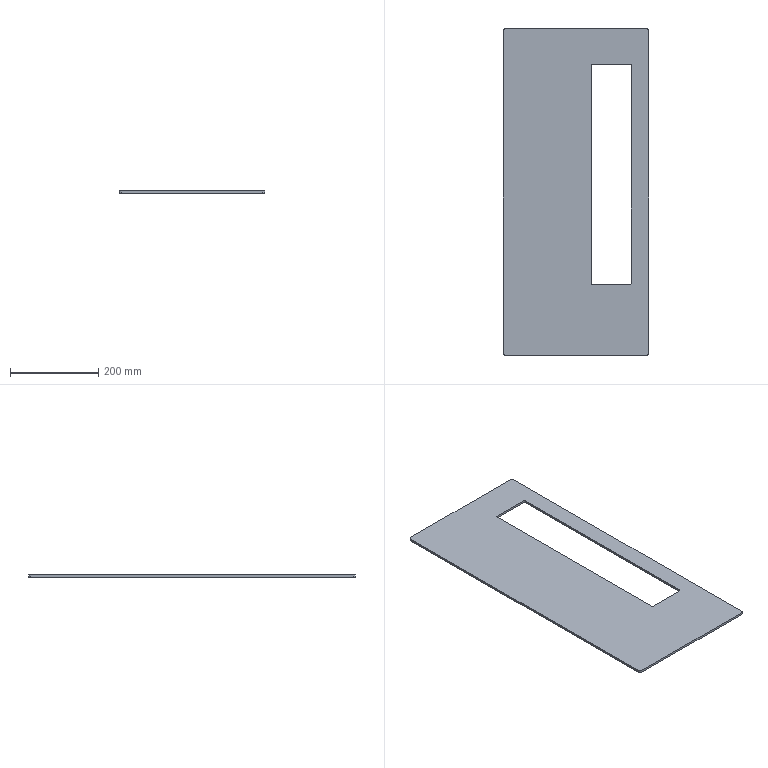Part | STEP file | 001-002-Face Plate-4 | 1 solid | 18 faces | box 330 x 740 x 5 mm | volume 995931 mm3 | plane 10 | cylinder 8 | commonest cylinder face diameters 6 x4 10 x4
STEP:
#1=CARTESIAN_POINT('',(0.,0.,0.));
#2=DIRECTION('',(0.,0.,1.));
#3=DIRECTION('',(1.,0.,0.));
#4=AXIS2_PLACEMENT_3D('',#1,#2,#3);
#5=CARTESIAN_POINT('',(165.,-365.,0.));
#6=VERTEX_POINT('',#5);
#7=CARTESIAN_POINT('',(165.,365.,0.));
#8=VERTEX_POINT('',#7);
#9=CARTESIAN_POINT('',(165.,-370.,0.));
#10=DIRECTION('',(0.,1.,0.));
#11=VECTOR('',#10,1.);
#12=LINE('',#9,#11);
#13=CARTESIAN_POINT('',(165.,-370.,5.));
#14=DIRECTION('',(-1.,0.,0.));
#15=DIRECTION('',(0.,0.,1.));
#16=AXIS2_PLACEMENT_3D('',#13,#14,#15);
#17=PLANE('',#16);
#18=CARTESIAN_POINT('',(-5.,0.));
#19=DIRECTION('',(0.,1.));
#20=VECTOR('',#19,1.);
#21=LINE('',#18,#20);
#22=(GEOMETRIC_REPRESENTATION_CONTEXT(2)PARAMETRIC_REPRESENTATION_CONTEXT()REPRESENTATION_CONTEXT('',''));
#23=DEFINITIONAL_REPRESENTATION('',(#21),#22);
#24=PCURVE('',#17,#23);
#25=CARTESIAN_POINT('',(0.,0.,0.));
#26=DIRECTION('',(0.,0.,-1.));
#27=DIRECTION('',(-1.,0.,0.));
#28=AXIS2_PLACEMENT_3D('',#25,#26,#27);
#29=PLANE('',#28);
#30=CARTESIAN_POINT('',(-165.,-370.));
#31=DIRECTION('',(0.,1.));
#32=VECTOR('',#31,1.);
#33=LINE('',#30,#32);
#34=(GEOMETRIC_REPRESENTATION_CONTEXT(2)PARAMETRIC_REPRESENTATION_CONTEXT()REPRESENTATION_CONTEXT('',''));
#35=DEFINITIONAL_REPRESENTATION('',(#33),#34);
#36=PCURVE('',#29,#35);
#37=SURFACE_CURVE('',#12,(#24,#36),.PCURVE_S1.);
#38=EDGE_CURVE('',#6,#8,#37,.T.);
#39=ORIENTED_EDGE('',*,*,#38,.T.);
#40=CARTESIAN_POINT('',(165.,365.,5.));
#41=VERTEX_POINT('',#40);
#42=CARTESIAN_POINT('',(165.,365.,5.));
#43=DIRECTION('',(0.,0.,1.));
#44=VECTOR('',#43,1.);
#45=LINE('',#42,#44);
#46=CARTESIAN_POINT('',(0.,735.));
#47=DIRECTION('',(1.,0.));
#48=VECTOR('',#47,1.);
#49=LINE('',#46,#48);
#50=(GEOMETRIC_REPRESENTATION_CONTEXT(2)PARAMETRIC_REPRESENTATION_CONTEXT()REPRESENTATION_CONTEXT('',''));
#51=DEFINITIONAL_REPRESENTATION('',(#49),#50);
#52=PCURVE('',#17,#51);
#53=CARTESIAN_POINT('',(160.,365.,5.));
#54=DIRECTION('',(0.,0.,-1.));
#55=DIRECTION('',(-1.,0.,0.));
#56=AXIS2_PLACEMENT_3D('',#53,#54,#55);
#57=CYLINDRICAL_SURFACE('',#56,5.);
#58=CARTESIAN_POINT('',(3.142,0.));
#59=DIRECTION('',(0.,-1.));
#60=VECTOR('',#59,1.);
#61=LINE('',#58,#60);
#62=(GEOMETRIC_REPRESENTATION_CONTEXT(2)PARAMETRIC_REPRESENTATION_CONTEXT()REPRESENTATION_CONTEXT('',''));
#63=DEFINITIONAL_REPRESENTATION('',(#61),#62);
#64=PCURVE('',#57,#63);
#65=SURFACE_CURVE('',#45,(#52,#64),.PCURVE_S1.);
#66=EDGE_CURVE('',#8,#41,#65,.T.);
#67=ORIENTED_EDGE('',*,*,#66,.T.);
#68=CARTESIAN_POINT('',(165.,-365.,5.));
#69=VERTEX_POINT('',#68);
#70=CARTESIAN_POINT('',(165.,-370.,5.));
#71=DIRECTION('',(0.,1.,0.));
#72=VECTOR('',#71,1.);
#73=LINE('',#70,#72);
#74=CARTESIAN_POINT('',(0.,0.));
#75=DIRECTION('',(0.,1.));
#76=VECTOR('',#75,1.);
#77=LINE('',#74,#76);
#78=(GEOMETRIC_REPRESENTATION_CONTEXT(2)PARAMETRIC_REPRESENTATION_CONTEXT()REPRESENTATION_CONTEXT('',''));
#79=DEFINITIONAL_REPRESENTATION('',(#77),#78);
#80=PCURVE('',#17,#79);
#81=CARTESIAN_POINT('',(0.,0.,5.));
#82=DIRECTION('',(0.,0.,-1.));
#83=DIRECTION('',(-1.,0.,0.));
#84=AXIS2_PLACEMENT_3D('',#81,#82,#83);
#85=PLANE('',#84);
#86=CARTESIAN_POINT('',(-165.,-370.));
#87=DIRECTION('',(0.,1.));
#88=VECTOR('',#87,1.);
#89=LINE('',#86,#88);
#90=(GEOMETRIC_REPRESENTATION_CONTEXT(2)PARAMETRIC_REPRESENTATION_CONTEXT()REPRESENTATION_CONTEXT('',''));
#91=DEFINITIONAL_REPRESENTATION('',(#89),#90);
#92=PCURVE('',#85,#91);
#93=SURFACE_CURVE('',#73,(#80,#92),.PCURVE_S1.);
#94=EDGE_CURVE('',#69,#41,#93,.T.);
#95=ORIENTED_EDGE('',*,*,#94,.F.);
#96=CARTESIAN_POINT('',(165.,-365.,5.));
#97=DIRECTION('',(0.,0.,-1.));
#98=VECTOR('',#97,1.);
#99=LINE('',#96,#98);
#100=CARTESIAN_POINT('',(0.,5.));
#101=DIRECTION('',(-1.,0.));
#102=VECTOR('',#101,1.);
#103=LINE('',#100,#102);
#104=(GEOMETRIC_REPRESENTATION_CONTEXT(2)PARAMETRIC_REPRESENTATION_CONTEXT()REPRESENTATION_CONTEXT('',''));
#105=DEFINITIONAL_REPRESENTATION('',(#103),#104);
#106=PCURVE('',#17,#105);
#107=CARTESIAN_POINT('',(160.,-365.,5.));
#108=DIRECTION('',(0.,0.,-1.));
#109=DIRECTION('',(-1.,0.,0.));
#110=AXIS2_PLACEMENT_3D('',#107,#108,#109);
#111=CYLINDRICAL_SURFACE('',#110,5.);
#112=CARTESIAN_POINT('',(3.142,0.));
#113=DIRECTION('',(0.,1.));
#114=VECTOR('',#113,1.);
#115=LINE('',#112,#114);
#116=(GEOMETRIC_REPRESENTATION_CONTEXT(2)PARAMETRIC_REPRESENTATION_CONTEXT()REPRESENTATION_CONTEXT('',''));
#117=DEFINITIONAL_REPRESENTATION('',(#115),#116);
#118=PCURVE('',#111,#117);
#119=SURFACE_CURVE('',#99,(#106,#118),.PCURVE_S1.);
#120=EDGE_CURVE('',#69,#6,#119,.T.);
#121=ORIENTED_EDGE('',*,*,#120,.T.);
#122=EDGE_LOOP('',(#39,#67,#95,#121));
#123=FACE_BOUND('',#122,.T.);
#124=ADVANCED_FACE('',(#123),#17,.F.);
#125=CARTESIAN_POINT('',(160.,370.,0.));
#126=VERTEX_POINT('',#125);
#127=CARTESIAN_POINT('',(-160.,370.,0.));
#128=VERTEX_POINT('',#127);
#129=CARTESIAN_POINT('',(-165.,370.,0.));
#130=DIRECTION('',(-1.,0.,0.));
#131=VECTOR('',#130,1.);
#132=LINE('',#129,#131);
#133=CARTESIAN_POINT('',(-165.,370.,5.));
#134=DIRECTION('',(0.,-1.,0.));
#135=DIRECTION('',(0.,0.,-1.));
#136=AXIS2_PLACEMENT_3D('',#133,#134,#135);
#137=PLANE('',#136);
#138=CARTESIAN_POINT('',(5.,0.));
#139=DIRECTION('',(0.,-1.));
#140=VECTOR('',#139,1.);
#141=LINE('',#138,#140);
#142=(GEOMETRIC_REPRESENTATION_CONTEXT(2)PARAMETRIC_REPRESENTATION_CONTEXT()REPRESENTATION_CONTEXT('',''));
#143=DEFINITIONAL_REPRESENTATION('',(#141),#142);
#144=PCURVE('',#137,#143);
#145=CARTESIAN_POINT('',(165.,370.));
#146=DIRECTION('',(1.,0.));
#147=VECTOR('',#146,1.);
#148=LINE('',#145,#147);
#149=(GEOMETRIC_REPRESENTATION_CONTEXT(2)PARAMETRIC_REPRESENTATION_CONTEXT()REPRESENTATION_CONTEXT('',''));
#150=DEFINITIONAL_REPRESENTATION('',(#148),#149);
#151=PCURVE('',#29,#150);
#152=SURFACE_CURVE('',#132,(#144,#151),.PCURVE_S1.);
#153=EDGE_CURVE('',#126,#128,#152,.T.);
#154=ORIENTED_EDGE('',*,*,#153,.T.);
#155=CARTESIAN_POINT('',(-160.,370.,5.));
#156=VERTEX_POINT('',#155);
#157=CARTESIAN_POINT('',(-160.,370.,5.));
#158=DIRECTION('',(0.,0.,1.));
#159=VECTOR('',#158,1.);
#160=LINE('',#157,#159);
#161=CARTESIAN_POINT('',(0.,5.));
#162=DIRECTION('',(-1.,0.));
#163=VECTOR('',#162,1.);
#164=LINE('',#161,#163);
#165=(GEOMETRIC_REPRESENTATION_CONTEXT(2)PARAMETRIC_REPRESENTATION_CONTEXT()REPRESENTATION_CONTEXT('',''));
#166=DEFINITIONAL_REPRESENTATION('',(#164),#165);
#167=PCURVE('',#137,#166);
#168=CARTESIAN_POINT('',(-160.,365.,5.));
#169=DIRECTION('',(0.,0.,-1.));
#170=DIRECTION('',(-1.,0.,0.));
#171=AXIS2_PLACEMENT_3D('',#168,#169,#170);
#172=CYLINDRICAL_SURFACE('',#171,5.);
#173=CARTESIAN_POINT('',(1.571,0.));
#174=DIRECTION('',(0.,-1.));
#175=VECTOR('',#174,1.);
#176=LINE('',#173,#175);
#177=(GEOMETRIC_REPRESENTATION_CONTEXT(2)PARAMETRIC_REPRESENTATION_CONTEXT()REPRESENTATION_CONTEXT('',''));
#178=DEFINITIONAL_REPRESENTATION('',(#176),#177);
#179=PCURVE('',#172,#178);
#180=SURFACE_CURVE('',#160,(#167,#179),.PCURVE_S1.);
#181=EDGE_CURVE('',#128,#156,#180,.T.);
#182=ORIENTED_EDGE('',*,*,#181,.T.);
#183=CARTESIAN_POINT('',(160.,370.,5.));
#184=VERTEX_POINT('',#183);
#185=CARTESIAN_POINT('',(-165.,370.,5.));
#186=DIRECTION('',(-1.,0.,0.));
#187=VECTOR('',#186,1.);
#188=LINE('',#185,#187);
#189=CARTESIAN_POINT('',(0.,0.));
#190=DIRECTION('',(0.,-1.));
#191=VECTOR('',#190,1.);
#192=LINE('',#189,#191);
#193=(GEOMETRIC_REPRESENTATION_CONTEXT(2)PARAMETRIC_REPRESENTATION_CONTEXT()REPRESENTATION_CONTEXT('',''));
#194=DEFINITIONAL_REPRESENTATION('',(#192),#193);
#195=PCURVE('',#137,#194);
#196=CARTESIAN_POINT('',(165.,370.));
#197=DIRECTION('',(1.,0.));
#198=VECTOR('',#197,1.);
#199=LINE('',#196,#198);
#200=(GEOMETRIC_REPRESENTATION_CONTEXT(2)PARAMETRIC_REPRESENTATION_CONTEXT()REPRESENTATION_CONTEXT('',''));
#201=DEFINITIONAL_REPRESENTATION('',(#199),#200);
#202=PCURVE('',#85,#201);
#203=SURFACE_CURVE('',#188,(#195,#202),.PCURVE_S1.);
#204=EDGE_CURVE('',#184,#156,#203,.T.);
#205=ORIENTED_EDGE('',*,*,#204,.F.);
#206=CARTESIAN_POINT('',(160.,370.,5.));
#207=DIRECTION('',(0.,0.,-1.));
#208=VECTOR('',#207,1.);
#209=LINE('',#206,#208);
#210=CARTESIAN_POINT('',(0.,325.));
#211=DIRECTION('',(1.,0.));
#212=VECTOR('',#211,1.);
#213=LINE('',#210,#212);
#214=(GEOMETRIC_REPRESENTATION_CONTEXT(2)PARAMETRIC_REPRESENTATION_CONTEXT()REPRESENTATION_CONTEXT('',''));
#215=DEFINITIONAL_REPRESENTATION('',(#213),#214);
#216=PCURVE('',#137,#215);
#217=CARTESIAN_POINT('',(1.571,0.));
#218=DIRECTION('',(0.,1.));
#219=VECTOR('',#218,1.);
#220=LINE('',#217,#219);
#221=(GEOMETRIC_REPRESENTATION_CONTEXT(2)PARAMETRIC_REPRESENTATION_CONTEXT()REPRESENTATION_CONTEXT('',''));
#222=DEFINITIONAL_REPRESENTATION('',(#220),#221);
#223=PCURVE('',#57,#222);
#224=SURFACE_CURVE('',#209,(#216,#223),.PCURVE_S1.);
#225=EDGE_CURVE('',#184,#126,#224,.T.);
#226=ORIENTED_EDGE('',*,*,#225,.T.);
#227=EDGE_LOOP('',(#154,#182,#205,#226));
#228=FACE_BOUND('',#227,.T.);
#229=ADVANCED_FACE('',(#228),#137,.F.);
#230=CARTESIAN_POINT('',(-165.,365.,0.));
#231=VERTEX_POINT('',#230);
#232=CARTESIAN_POINT('',(-165.,-365.,0.));
#233=VERTEX_POINT('',#232);
#234=CARTESIAN_POINT('',(-165.,-370.,0.));
#235=DIRECTION('',(0.,-1.,0.));
#236=VECTOR('',#235,1.);
#237=LINE('',#234,#236);
#238=CARTESIAN_POINT('',(-165.,-370.,5.));
#239=DIRECTION('',(1.,0.,0.));
#240=DIRECTION('',(0.,0.,-1.));
#241=AXIS2_PLACEMENT_3D('',#238,#239,#240);
#242=PLANE('',#241);
#243=CARTESIAN_POINT('',(5.,0.));
#244=DIRECTION('',(0.,-1.));
#245=VECTOR('',#244,1.);
#246=LINE('',#243,#245);
#247=(GEOMETRIC_REPRESENTATION_CONTEXT(2)PARAMETRIC_REPRESENTATION_CONTEXT()REPRESENTATION_CONTEXT('',''));
#248=DEFINITIONAL_REPRESENTATION('',(#246),#247);
#249=PCURVE('',#242,#248);
#250=CARTESIAN_POINT('',(165.,-370.));
#251=DIRECTION('',(0.,-1.));
#252=VECTOR('',#251,1.);
#253=LINE('',#250,#252);
#254=(GEOMETRIC_REPRESENTATION_CONTEXT(2)PARAMETRIC_REPRESENTATION_CONTEXT()REPRESENTATION_CONTEXT('',''));
#255=DEFINITIONAL_REPRESENTATION('',(#253),#254);
#256=PCURVE('',#29,#255);
#257=SURFACE_CURVE('',#237,(#249,#256),.PCURVE_S1.);
#258=EDGE_CURVE('',#231,#233,#257,.T.);
#259=ORIENTED_EDGE('',*,*,#258,.T.);
#260=CARTESIAN_POINT('',(-165.,-365.,5.));
#261=VERTEX_POINT('',#260);
#262=CARTESIAN_POINT('',(-165.,-365.,5.));
#263=DIRECTION('',(0.,0.,1.));
#264=VECTOR('',#263,1.);
#265=LINE('',#262,#264);
#266=CARTESIAN_POINT('',(0.,5.));
#267=DIRECTION('',(-1.,0.));
#268=VECTOR('',#267,1.);
#269=LINE('',#266,#268);
#270=(GEOMETRIC_REPRESENTATION_CONTEXT(2)PARAMETRIC_REPRESENTATION_CONTEXT()REPRESENTATION_CONTEXT('',''));
#271=DEFINITIONAL_REPRESENTATION('',(#269),#270);
#272=PCURVE('',#242,#271);
#273=CARTESIAN_POINT('',(-160.,-365.,5.));
#274=DIRECTION('',(0.,0.,-1.));
#275=DIRECTION('',(-1.,0.,0.));
#276=AXIS2_PLACEMENT_3D('',#273,#274,#275);
#277=CYLINDRICAL_SURFACE('',#276,5.);
#278=CARTESIAN_POINT('',(6.283,0.));
#279=DIRECTION('',(0.,-1.));
#280=VECTOR('',#279,1.);
#281=LINE('',#278,#280);
#282=(GEOMETRIC_REPRESENTATION_CONTEXT(2)PARAMETRIC_REPRESENTATION_CONTEXT()REPRESENTATION_CONTEXT('',''));
#283=DEFINITIONAL_REPRESENTATION('',(#281),#282);
#284=PCURVE('',#277,#283);
#285=SURFACE_CURVE('',#265,(#272,#284),.PCURVE_S1.);
#286=EDGE_CURVE('',#233,#261,#285,.T.);
#287=ORIENTED_EDGE('',*,*,#286,.T.);
#288=CARTESIAN_POINT('',(-165.,365.,5.));
#289=VERTEX_POINT('',#288);
#290=CARTESIAN_POINT('',(-165.,-370.,5.));
#291=DIRECTION('',(0.,-1.,0.));
#292=VECTOR('',#291,1.);
#293=LINE('',#290,#292);
#294=CARTESIAN_POINT('',(0.,0.));
#295=DIRECTION('',(0.,-1.));
#296=VECTOR('',#295,1.);
#297=LINE('',#294,#296);
#298=(GEOMETRIC_REPRESENTATION_CONTEXT(2)PARAMETRIC_REPRESENTATION_CONTEXT()REPRESENTATION_CONTEXT('',''));
#299=DEFINITIONAL_REPRESENTATION('',(#297),#298);
#300=PCURVE('',#242,#299);
#301=CARTESIAN_POINT('',(165.,-370.));
#302=DIRECTION('',(0.,-1.));
#303=VECTOR('',#302,1.);
#304=LINE('',#301,#303);
#305=(GEOMETRIC_REPRESENTATION_CONTEXT(2)PARAMETRIC_REPRESENTATION_CONTEXT()REPRESENTATION_CONTEXT('',''));
#306=DEFINITIONAL_REPRESENTATION('',(#304),#305);
#307=PCURVE('',#85,#306);
#308=SURFACE_CURVE('',#293,(#300,#307),.PCURVE_S1.);
#309=EDGE_CURVE('',#289,#261,#308,.T.);
#310=ORIENTED_EDGE('',*,*,#309,.F.);
#311=CARTESIAN_POINT('',(-165.,365.,5.));
#312=DIRECTION('',(0.,0.,-1.));
#313=VECTOR('',#312,1.);
#314=LINE('',#311,#313);
#315=CARTESIAN_POINT('',(0.,735.));
#316=DIRECTION('',(1.,0.));
#317=VECTOR('',#316,1.);
#318=LINE('',#315,#317);
#319=(GEOMETRIC_REPRESENTATION_CONTEXT(2)PARAMETRIC_REPRESENTATION_CONTEXT()REPRESENTATION_CONTEXT('',''));
#320=DEFINITIONAL_REPRESENTATION('',(#318),#319);
#321=PCURVE('',#242,#320);
#322=CARTESIAN_POINT('',(0.,0.));
#323=DIRECTION('',(0.,1.));
#324=VECTOR('',#323,1.);
#325=LINE('',#322,#324);
#326=(GEOMETRIC_REPRESENTATION_CONTEXT(2)PARAMETRIC_REPRESENTATION_CONTEXT()REPRESENTATION_CONTEXT('',''));
#327=DEFINITIONAL_REPRESENTATION('',(#325),#326);
#328=PCURVE('',#172,#327);
#329=SURFACE_CURVE('',#314,(#321,#328),.PCURVE_S1.);
#330=EDGE_CURVE('',#289,#231,#329,.T.);
#331=ORIENTED_EDGE('',*,*,#330,.T.);
#332=EDGE_LOOP('',(#259,#287,#310,#331));
#333=FACE_BOUND('',#332,.T.);
#334=ADVANCED_FACE('',(#333),#242,.F.);
#335=CARTESIAN_POINT('',(-160.,-370.,5.));
#336=VERTEX_POINT('',#335);
#337=CARTESIAN_POINT('',(160.,-370.,5.));
#338=VERTEX_POINT('',#337);
#339=CARTESIAN_POINT('',(-165.,-370.,5.));
#340=DIRECTION('',(1.,0.,0.));
#341=VECTOR('',#340,1.);
#342=LINE('',#339,#341);
#343=CARTESIAN_POINT('',(-165.,-370.,5.));
#344=DIRECTION('',(0.,1.,0.));
#345=DIRECTION('',(0.,0.,1.));
#346=AXIS2_PLACEMENT_3D('',#343,#344,#345);
#347=PLANE('',#346);
#348=CARTESIAN_POINT('',(0.,0.));
#349=DIRECTION('',(0.,1.));
#350=VECTOR('',#349,1.);
#351=LINE('',#348,#350);
#352=(GEOMETRIC_REPRESENTATION_CONTEXT(2)PARAMETRIC_REPRESENTATION_CONTEXT()REPRESENTATION_CONTEXT('',''));
#353=DEFINITIONAL_REPRESENTATION('',(#351),#352);
#354=PCURVE('',#347,#353);
#355=CARTESIAN_POINT('',(165.,-370.));
#356=DIRECTION('',(-1.,0.));
#357=VECTOR('',#356,1.);
#358=LINE('',#355,#357);
#359=(GEOMETRIC_REPRESENTATION_CONTEXT(2)PARAMETRIC_REPRESENTATION_CONTEXT()REPRESENTATION_CONTEXT('',''));
#360=DEFINITIONAL_REPRESENTATION('',(#358),#359);
#361=PCURVE('',#85,#360);
#362=SURFACE_CURVE('',#342,(#354,#361),.PCURVE_S1.);
#363=EDGE_CURVE('',#336,#338,#362,.T.);
#364=ORIENTED_EDGE('',*,*,#363,.F.);
#365=CARTESIAN_POINT('',(-160.,-370.,0.));
#366=VERTEX_POINT('',#365);
#367=CARTESIAN_POINT('',(-160.,-370.,5.));
#368=DIRECTION('',(0.,0.,-1.));
#369=VECTOR('',#368,1.);
#370=LINE('',#367,#369);
#371=CARTESIAN_POINT('',(0.,5.));
#372=DIRECTION('',(-1.,0.));
#373=VECTOR('',#372,1.);
#374=LINE('',#371,#373);
#375=(GEOMETRIC_REPRESENTATION_CONTEXT(2)PARAMETRIC_REPRESENTATION_CONTEXT()REPRESENTATION_CONTEXT('',''));
#376=DEFINITIONAL_REPRESENTATION('',(#374),#375);
#377=PCURVE('',#347,#376);
#378=CARTESIAN_POINT('',(4.712,0.));
#379=DIRECTION('',(0.,1.));
#380=VECTOR('',#379,1.);
#381=LINE('',#378,#380);
#382=(GEOMETRIC_REPRESENTATION_CONTEXT(2)PARAMETRIC_REPRESENTATION_CONTEXT()REPRESENTATION_CONTEXT('',''));
#383=DEFINITIONAL_REPRESENTATION('',(#381),#382);
#384=PCURVE('',#277,#383);
#385=SURFACE_CURVE('',#370,(#377,#384),.PCURVE_S1.);
#386=EDGE_CURVE('',#336,#366,#385,.T.);
#387=ORIENTED_EDGE('',*,*,#386,.T.);
#388=CARTESIAN_POINT('',(160.,-370.,0.));
#389=VERTEX_POINT('',#388);
#390=CARTESIAN_POINT('',(-165.,-370.,0.));
#391=DIRECTION('',(1.,0.,0.));
#392=VECTOR('',#391,1.);
#393=LINE('',#390,#392);
#394=CARTESIAN_POINT('',(-5.,0.));
#395=DIRECTION('',(0.,1.));
#396=VECTOR('',#395,1.);
#397=LINE('',#394,#396);
#398=(GEOMETRIC_REPRESENTATION_CONTEXT(2)PARAMETRIC_REPRESENTATION_CONTEXT()REPRESENTATION_CONTEXT('',''));
#399=DEFINITIONAL_REPRESENTATION('',(#397),#398);
#400=PCURVE('',#347,#399);
#401=CARTESIAN_POINT('',(165.,-370.));
#402=DIRECTION('',(-1.,0.));
#403=VECTOR('',#402,1.);
#404=LINE('',#401,#403);
#405=(GEOMETRIC_REPRESENTATION_CONTEXT(2)PARAMETRIC_REPRESENTATION_CONTEXT()REPRESENTATION_CONTEXT('',''));
#406=DEFINITIONAL_REPRESENTATION('',(#404),#405);
#407=PCURVE('',#29,#406);
#408=SURFACE_CURVE('',#393,(#400,#407),.PCURVE_S1.);
#409=EDGE_CURVE('',#366,#389,#408,.T.);
#410=ORIENTED_EDGE('',*,*,#409,.T.);
#411=CARTESIAN_POINT('',(160.,-370.,5.));
#412=DIRECTION('',(0.,0.,1.));
#413=VECTOR('',#412,1.);
#414=LINE('',#411,#413);
#415=CARTESIAN_POINT('',(0.,325.));
#416=DIRECTION('',(1.,0.));
#417=VECTOR('',#416,1.);
#418=LINE('',#415,#417);
#419=(GEOMETRIC_REPRESENTATION_CONTEXT(2)PARAMETRIC_REPRESENTATION_CONTEXT()REPRESENTATION_CONTEXT('',''));
#420=DEFINITIONAL_REPRESENTATION('',(#418),#419);
#421=PCURVE('',#347,#420);
#422=CARTESIAN_POINT('',(4.712,0.));
#423=DIRECTION('',(0.,-1.));
#424=VECTOR('',#423,1.);
#425=LINE('',#422,#424);
#426=(GEOMETRIC_REPRESENTATION_CONTEXT(2)PARAMETRIC_REPRESENTATION_CONTEXT()REPRESENTATION_CONTEXT('',''));
#427=DEFINITIONAL_REPRESENTATION('',(#425),#426);
#428=PCURVE('',#111,#427);
#429=SURFACE_CURVE('',#414,(#421,#428),.PCURVE_S1.);
#430=EDGE_CURVE('',#389,#338,#429,.T.);
#431=ORIENTED_EDGE('',*,*,#430,.T.);
#432=EDGE_LOOP('',(#364,#387,#410,#431));
#433=FACE_BOUND('',#432,.T.);
#434=ADVANCED_FACE('',(#433),#347,.F.);
#435=CARTESIAN_POINT('',(35.,-207.,5.));
#436=VERTEX_POINT('',#435);
#437=CARTESIAN_POINT('',(35.,287.,5.));
#438=VERTEX_POINT('',#437);
#439=CARTESIAN_POINT('',(35.,0.,5.));
#440=DIRECTION('',(0.,1.,0.));
#441=VECTOR('',#440,1.);
#442=LINE('',#439,#441);
#443=CARTESIAN_POINT('',(-35.,0.));
#444=DIRECTION('',(0.,1.));
#445=VECTOR('',#444,1.);
#446=LINE('',#443,#445);
#447=(GEOMETRIC_REPRESENTATION_CONTEXT(2)PARAMETRIC_REPRESENTATION_CONTEXT()REPRESENTATION_CONTEXT('',''));
#448=DEFINITIONAL_REPRESENTATION('',(#446),#447);
#449=PCURVE('',#85,#448);
#450=CARTESIAN_POINT('',(35.,-210.,10.));
#451=DIRECTION('',(-1.,0.,0.));
#452=DIRECTION('',(0.,-1.,0.));
#453=AXIS2_PLACEMENT_3D('',#450,#451,#452);
#454=PLANE('',#453);
#455=CARTESIAN_POINT('',(-210.,-5.));
#456=DIRECTION('',(-1.,0.));
#457=VECTOR('',#456,1.);
#458=LINE('',#455,#457);
#459=(GEOMETRIC_REPRESENTATION_CONTEXT(2)PARAMETRIC_REPRESENTATION_CONTEXT()REPRESENTATION_CONTEXT('',''));
#460=DEFINITIONAL_REPRESENTATION('',(#458),#459);
#461=PCURVE('',#454,#460);
#462=SURFACE_CURVE('',#442,(#449,#461),.PCURVE_S1.);
#463=EDGE_CURVE('',#436,#438,#462,.T.);
#464=ORIENTED_EDGE('',*,*,#463,.T.);
#465=CARTESIAN_POINT('',(38.,290.,5.));
#466=VERTEX_POINT('',#465);
#467=CARTESIAN_POINT('',(38.,287.,5.));
#468=DIRECTION('',(0.,0.,-1.));
#469=DIRECTION('',(-1.,0.,0.));
#470=AXIS2_PLACEMENT_3D('',#467,#468,#469);
#471=CIRCLE('',#470,3.);
#472=CARTESIAN_POINT('',(-38.,287.));
#473=DIRECTION('',(1.,0.));
#474=AXIS2_PLACEMENT_2D('',#472,#473);
#475=CIRCLE('',#474,3.);
#476=(GEOMETRIC_REPRESENTATION_CONTEXT(2)PARAMETRIC_REPRESENTATION_CONTEXT()REPRESENTATION_CONTEXT('',''));
#477=DEFINITIONAL_REPRESENTATION('',(#475),#476);
#478=PCURVE('',#85,#477);
#479=CARTESIAN_POINT('',(38.,287.,10.));
#480=DIRECTION('',(0.,0.,1.));
#481=DIRECTION('',(1.,0.,0.));
#482=AXIS2_PLACEMENT_3D('',#479,#480,#481);
#483=CYLINDRICAL_SURFACE('',#482,3.);
#484=CARTESIAN_POINT('',(3.142,-5.));
#485=DIRECTION('',(-1.,0.));
#486=VECTOR('',#485,1.);
#487=LINE('',#484,#486);
#488=(GEOMETRIC_REPRESENTATION_CONTEXT(2)PARAMETRIC_REPRESENTATION_CONTEXT()REPRESENTATION_CONTEXT('',''));
#489=DEFINITIONAL_REPRESENTATION('',(#487),#488);
#490=PCURVE('',#483,#489);
#491=SURFACE_CURVE('',#471,(#478,#490),.PCURVE_S1.);
#492=EDGE_CURVE('',#438,#466,#491,.T.);
#493=ORIENTED_EDGE('',*,*,#492,.T.);
#494=CARTESIAN_POINT('',(122.,290.,5.));
#495=VERTEX_POINT('',#494);
#496=CARTESIAN_POINT('',(0.,290.,5.));
#497=DIRECTION('',(1.,0.,0.));
#498=VECTOR('',#497,1.);
#499=LINE('',#496,#498);
#500=CARTESIAN_POINT('',(0.,290.));
#501=DIRECTION('',(-1.,0.));
#502=VECTOR('',#501,1.);
#503=LINE('',#500,#502);
#504=(GEOMETRIC_REPRESENTATION_CONTEXT(2)PARAMETRIC_REPRESENTATION_CONTEXT()REPRESENTATION_CONTEXT('',''));
#505=DEFINITIONAL_REPRESENTATION('',(#503),#504);
#506=PCURVE('',#85,#505);
#507=CARTESIAN_POINT('',(35.,290.,10.));
#508=DIRECTION('',(0.,1.,0.));
#509=DIRECTION('',(0.,0.,1.));
#510=AXIS2_PLACEMENT_3D('',#507,#508,#509);
#511=PLANE('',#510);
#512=CARTESIAN_POINT('',(-5.,-35.));
#513=DIRECTION('',(0.,1.));
#514=VECTOR('',#513,1.);
#515=LINE('',#512,#514);
#516=(GEOMETRIC_REPRESENTATION_CONTEXT(2)PARAMETRIC_REPRESENTATION_CONTEXT()REPRESENTATION_CONTEXT('',''));
#517=DEFINITIONAL_REPRESENTATION('',(#515),#516);
#518=PCURVE('',#511,#517);
#519=SURFACE_CURVE('',#499,(#506,#518),.PCURVE_S1.);
#520=EDGE_CURVE('',#466,#495,#519,.T.);
#521=ORIENTED_EDGE('',*,*,#520,.T.);
#522=CARTESIAN_POINT('',(125.,287.,5.));
#523=VERTEX_POINT('',#522);
#524=CARTESIAN_POINT('',(122.,287.,5.));
#525=DIRECTION('',(0.,0.,-1.));
#526=DIRECTION('',(-1.,0.,0.));
#527=AXIS2_PLACEMENT_3D('',#524,#525,#526);
#528=CIRCLE('',#527,3.);
#529=CARTESIAN_POINT('',(-122.,287.));
#530=DIRECTION('',(1.,0.));
#531=AXIS2_PLACEMENT_2D('',#529,#530);
#532=CIRCLE('',#531,3.);
#533=(GEOMETRIC_REPRESENTATION_CONTEXT(2)PARAMETRIC_REPRESENTATION_CONTEXT()REPRESENTATION_CONTEXT('',''));
#534=DEFINITIONAL_REPRESENTATION('',(#532),#533);
#535=PCURVE('',#85,#534);
#536=CARTESIAN_POINT('',(122.,287.,10.));
#537=DIRECTION('',(0.,0.,1.));
#538=DIRECTION('',(1.,0.,0.));
#539=AXIS2_PLACEMENT_3D('',#536,#537,#538);
#540=CYLINDRICAL_SURFACE('',#539,3.);
#541=CARTESIAN_POINT('',(3.142,-5.));
#542=DIRECTION('',(-1.,0.));
#543=VECTOR('',#542,1.);
#544=LINE('',#541,#543);
#545=(GEOMETRIC_REPRESENTATION_CONTEXT(2)PARAMETRIC_REPRESENTATION_CONTEXT()REPRESENTATION_CONTEXT('',''));
#546=DEFINITIONAL_REPRESENTATION('',(#544),#545);
#547=PCURVE('',#540,#546);
#548=SURFACE_CURVE('',#528,(#535,#547),.PCURVE_S1.);
#549=EDGE_CURVE('',#495,#523,#548,.T.);
#550=ORIENTED_EDGE('',*,*,#549,.T.);
#551=CARTESIAN_POINT('',(125.,-207.,5.));
#552=VERTEX_POINT('',#551);
#553=CARTESIAN_POINT('',(125.,0.,5.));
#554=DIRECTION('',(0.,-1.,0.));
#555=VECTOR('',#554,1.);
#556=LINE('',#553,#555);
#557=CARTESIAN_POINT('',(-125.,0.));
#558=DIRECTION('',(0.,-1.));
#559=VECTOR('',#558,1.);
#560=LINE('',#557,#559);
#561=(GEOMETRIC_REPRESENTATION_CONTEXT(2)PARAMETRIC_REPRESENTATION_CONTEXT()REPRESENTATION_CONTEXT('',''));
#562=DEFINITIONAL_REPRESENTATION('',(#560),#561);
#563=PCURVE('',#85,#562);
#564=CARTESIAN_POINT('',(125.,-210.,10.));
#565=DIRECTION('',(1.,0.,0.));
#566=DIRECTION('',(0.,0.,-1.));
#567=AXIS2_PLACEMENT_3D('',#564,#565,#566);
#568=PLANE('',#567);
#569=CARTESIAN_POINT('',(5.,210.));
#570=DIRECTION('',(0.,-1.));
#571=VECTOR('',#570,1.);
#572=LINE('',#569,#571);
#573=(GEOMETRIC_REPRESENTATION_CONTEXT(2)PARAMETRIC_REPRESENTATION_CONTEXT()REPRESENTATION_CONTEXT('',''));
#574=DEFINITIONAL_REPRESENTATION('',(#572),#573);
#575=PCURVE('',#568,#574);
#576=SURFACE_CURVE('',#556,(#563,#575),.PCURVE_S1.);
#577=EDGE_CURVE('',#523,#552,#576,.T.);
#578=ORIENTED_EDGE('',*,*,#577,.T.);
#579=CARTESIAN_POINT('',(122.,-210.,5.));
#580=VERTEX_POINT('',#579);
#581=CARTESIAN_POINT('',(122.,-207.,5.));
#582=DIRECTION('',(0.,0.,-1.));
#583=DIRECTION('',(-1.,0.,0.));
#584=AXIS2_PLACEMENT_3D('',#581,#582,#583);
#585=CIRCLE('',#584,3.);
#586=CARTESIAN_POINT('',(-122.,-207.));
#587=DIRECTION('',(1.,0.));
#588=AXIS2_PLACEMENT_2D('',#586,#587);
#589=CIRCLE('',#588,3.);
#590=(GEOMETRIC_REPRESENTATION_CONTEXT(2)PARAMETRIC_REPRESENTATION_CONTEXT()REPRESENTATION_CONTEXT('',''));
#591=DEFINITIONAL_REPRESENTATION('',(#589),#590);
#592=PCURVE('',#85,#591);
#593=CARTESIAN_POINT('',(122.,-207.,10.));
#594=DIRECTION('',(0.,0.,1.));
#595=DIRECTION('',(1.,0.,0.));
#596=AXIS2_PLACEMENT_3D('',#593,#594,#595);
#597=CYLINDRICAL_SURFACE('',#596,3.);
#598=CARTESIAN_POINT('',(9.425,-5.));
#599=DIRECTION('',(-1.,0.));
#600=VECTOR('',#599,1.);
#601=LINE('',#598,#600);
#602=(GEOMETRIC_REPRESENTATION_CONTEXT(2)PARAMETRIC_REPRESENTATION_CONTEXT()REPRESENTATION_CONTEXT('',''));
#603=DEFINITIONAL_REPRESENTATION('',(#601),#602);
#604=PCURVE('',#597,#603);
#605=SURFACE_CURVE('',#585,(#592,#604),.PCURVE_S1.);
#606=EDGE_CURVE('',#552,#580,#605,.T.);
#607=ORIENTED_EDGE('',*,*,#606,.T.);
#608=CARTESIAN_POINT('',(38.,-210.,5.));
#609=VERTEX_POINT('',#608);
#610=CARTESIAN_POINT('',(0.,-210.,5.));
#611=DIRECTION('',(-1.,0.,0.));
#612=VECTOR('',#611,1.);
#613=LINE('',#610,#612);
#614=CARTESIAN_POINT('',(0.,-210.));
#615=DIRECTION('',(1.,0.));
#616=VECTOR('',#615,1.);
#617=LINE('',#614,#616);
#618=(GEOMETRIC_REPRESENTATION_CONTEXT(2)PARAMETRIC_REPRESENTATION_CONTEXT()REPRESENTATION_CONTEXT('',''));
#619=DEFINITIONAL_REPRESENTATION('',(#617),#618);
#620=PCURVE('',#85,#619);
#621=CARTESIAN_POINT('',(35.,-210.,10.));
#622=DIRECTION('',(0.,-1.,0.));
#623=DIRECTION('',(1.,0.,0.));
#624=AXIS2_PLACEMENT_3D('',#621,#622,#623);
#625=PLANE('',#624);
#626=CARTESIAN_POINT('',(-35.,-5.));
#627=DIRECTION('',(-1.,0.));
#628=VECTOR('',#627,1.);
#629=LINE('',#626,#628);
#630=(GEOMETRIC_REPRESENTATION_CONTEXT(2)PARAMETRIC_REPRESENTATION_CONTEXT()REPRESENTATION_CONTEXT('',''));
#631=DEFINITIONAL_REPRESENTATION('',(#629),#630);
#632=PCURVE('',#625,#631);
#633=SURFACE_CURVE('',#613,(#620,#632),.PCURVE_S1.);
#634=EDGE_CURVE('',#580,#609,#633,.T.);
#635=ORIENTED_EDGE('',*,*,#634,.T.);
#636=CARTESIAN_POINT('',(38.,-207.,5.));
#637=DIRECTION('',(0.,0.,-1.));
#638=DIRECTION('',(-1.,0.,0.));
#639=AXIS2_PLACEMENT_3D('',#636,#637,#638);
#640=CIRCLE('',#639,3.);
#641=CARTESIAN_POINT('',(-38.,-207.));
#642=DIRECTION('',(1.,0.));
#643=AXIS2_PLACEMENT_2D('',#641,#642);
#644=CIRCLE('',#643,3.);
#645=(GEOMETRIC_REPRESENTATION_CONTEXT(2)PARAMETRIC_REPRESENTATION_CONTEXT()REPRESENTATION_CONTEXT('',''));
#646=DEFINITIONAL_REPRESENTATION('',(#644),#645);
#647=PCURVE('',#85,#646);
#648=CARTESIAN_POINT('',(38.,-207.,10.));
#649=DIRECTION('',(0.,0.,1.));
#650=DIRECTION('',(1.,0.,0.));
#651=AXIS2_PLACEMENT_3D('',#648,#649,#650);
#652=CYLINDRICAL_SURFACE('',#651,3.);
#653=CARTESIAN_POINT('',(9.425,-5.));
#654=DIRECTION('',(-1.,0.));
#655=VECTOR('',#654,1.);
#656=LINE('',#653,#655);
#657=(GEOMETRIC_REPRESENTATION_CONTEXT(2)PARAMETRIC_REPRESENTATION_CONTEXT()REPRESENTATION_CONTEXT('',''));
#658=DEFINITIONAL_REPRESENTATION('',(#656),#657);
#659=PCURVE('',#652,#658);
#660=SURFACE_CURVE('',#640,(#647,#659),.PCURVE_S1.);
#661=EDGE_CURVE('',#609,#436,#660,.T.);
#662=ORIENTED_EDGE('',*,*,#661,.T.);
#663=EDGE_LOOP('',(#464,#493,#521,#550,#578,#607,#635,#662));
#664=FACE_BOUND('',#663,.T.);
#665=ORIENTED_EDGE('',*,*,#309,.T.);
#666=CARTESIAN_POINT('',(-160.,-365.,5.));
#667=DIRECTION('',(0.,0.,1.));
#668=DIRECTION('',(-1.,0.,0.));
#669=AXIS2_PLACEMENT_3D('',#666,#667,#668);
#670=CIRCLE('',#669,5.);
#671=CARTESIAN_POINT('',(165.,-365.));
#672=CARTESIAN_POINT('',(165.,-373.66));
#673=CARTESIAN_POINT('',(157.5,-369.33));
#674=CARTESIAN_POINT('',(150.,-365.));
#675=CARTESIAN_POINT('',(157.5,-360.67));
#676=CARTESIAN_POINT('',(165.,-356.34));
#677=CARTESIAN_POINT('',(165.,-365.));
#678=(BOUNDED_CURVE()B_SPLINE_CURVE(2,(#671,#672,#673,#674,#675,#676,#677),.UNSPECIFIED.,.T.,.F.)B_SPLINE_CURVE_WITH_KNOTS((1,2,2,2,2,1),(-2.094,0.,2.094,4.189,6.283,8.378),.UNSPECIFIED.)CURVE()GEOMETRIC_REPRESENTATION_ITEM()RATIONAL_B_SPLINE_CURVE((1.,0.5,1.,0.5,1.,0.5,1.))REPRESENTATION_ITEM(''));
#679=(GEOMETRIC_REPRESENTATION_CONTEXT(2)PARAMETRIC_REPRESENTATION_CONTEXT()REPRESENTATION_CONTEXT('',''));
#680=DEFINITIONAL_REPRESENTATION('',(#678),#679);
#681=PCURVE('',#85,#680);
#682=CARTESIAN_POINT('',(6.283,0.));
#683=DIRECTION('',(-1.,0.));
#684=VECTOR('',#683,1.);
#685=LINE('',#682,#684);
#686=(GEOMETRIC_REPRESENTATION_CONTEXT(2)PARAMETRIC_REPRESENTATION_CONTEXT()REPRESENTATION_CONTEXT('',''));
#687=DEFINITIONAL_REPRESENTATION('',(#685),#686);
#688=PCURVE('',#277,#687);
#689=SURFACE_CURVE('',#670,(#681,#688),.PCURVE_S1.);
#690=EDGE_CURVE('',#261,#336,#689,.T.);
#691=ORIENTED_EDGE('',*,*,#690,.T.);
#692=ORIENTED_EDGE('',*,*,#363,.T.);
#693=CARTESIAN_POINT('',(160.,-365.,5.));
#694=DIRECTION('',(0.,0.,1.));
#695=DIRECTION('',(-1.,0.,0.));
#696=AXIS2_PLACEMENT_3D('',#693,#694,#695);
#697=CIRCLE('',#696,5.);
#698=CARTESIAN_POINT('',(-155.,-365.));
#699=CARTESIAN_POINT('',(-155.,-373.66));
#700=CARTESIAN_POINT('',(-162.5,-369.33));
#701=CARTESIAN_POINT('',(-170.,-365.));
#702=CARTESIAN_POINT('',(-162.5,-360.67));
#703=CARTESIAN_POINT('',(-155.,-356.34));
#704=CARTESIAN_POINT('',(-155.,-365.));
#705=(BOUNDED_CURVE()B_SPLINE_CURVE(2,(#698,#699,#700,#701,#702,#703,#704),.UNSPECIFIED.,.T.,.F.)B_SPLINE_CURVE_WITH_KNOTS((1,2,2,2,2,1),(-2.094,0.,2.094,4.189,6.283,8.378),.UNSPECIFIED.)CURVE()GEOMETRIC_REPRESENTATION_ITEM()RATIONAL_B_SPLINE_CURVE((1.,0.5,1.,0.5,1.,0.5,1.))REPRESENTATION_ITEM(''));
#706=(GEOMETRIC_REPRESENTATION_CONTEXT(2)PARAMETRIC_REPRESENTATION_CONTEXT()REPRESENTATION_CONTEXT('',''));
#707=DEFINITIONAL_REPRESENTATION('',(#705),#706);
#708=PCURVE('',#85,#707);
#709=CARTESIAN_POINT('',(6.283,0.));
#710=DIRECTION('',(-1.,0.));
#711=VECTOR('',#710,1.);
#712=LINE('',#709,#711);
#713=(GEOMETRIC_REPRESENTATION_CONTEXT(2)PARAMETRIC_REPRESENTATION_CONTEXT()REPRESENTATION_CONTEXT('',''));
#714=DEFINITIONAL_REPRESENTATION('',(#712),#713);
#715=PCURVE('',#111,#714);
#716=SURFACE_CURVE('',#697,(#708,#715),.PCURVE_S1.);
#717=EDGE_CURVE('',#338,#69,#716,.T.);
#718=ORIENTED_EDGE('',*,*,#717,.T.);
#719=ORIENTED_EDGE('',*,*,#94,.T.);
#720=CARTESIAN_POINT('',(160.,365.,5.));
#721=DIRECTION('',(0.,0.,1.));
#722=DIRECTION('',(-1.,0.,0.));
#723=AXIS2_PLACEMENT_3D('',#720,#721,#722);
#724=CIRCLE('',#723,5.);
#725=CARTESIAN_POINT('',(-155.,365.));
#726=CARTESIAN_POINT('',(-155.,356.34));
#727=CARTESIAN_POINT('',(-162.5,360.67));
#728=CARTESIAN_POINT('',(-170.,365.));
#729=CARTESIAN_POINT('',(-162.5,369.33));
#730=CARTESIAN_POINT('',(-155.,373.66));
#731=CARTESIAN_POINT('',(-155.,365.));
#732=(BOUNDED_CURVE()B_SPLINE_CURVE(2,(#725,#726,#727,#728,#729,#730,#731),.UNSPECIFIED.,.T.,.F.)B_SPLINE_CURVE_WITH_KNOTS((1,2,2,2,2,1),(-2.094,0.,2.094,4.189,6.283,8.378),.UNSPECIFIED.)CURVE()GEOMETRIC_REPRESENTATION_ITEM()RATIONAL_B_SPLINE_CURVE((1.,0.5,1.,0.5,1.,0.5,1.))REPRESENTATION_ITEM(''));
#733=(GEOMETRIC_REPRESENTATION_CONTEXT(2)PARAMETRIC_REPRESENTATION_CONTEXT()REPRESENTATION_CONTEXT('',''));
#734=DEFINITIONAL_REPRESENTATION('',(#732),#733);
#735=PCURVE('',#85,#734);
#736=CARTESIAN_POINT('',(6.283,0.));
#737=DIRECTION('',(-1.,0.));
#738=VECTOR('',#737,1.);
#739=LINE('',#736,#738);
#740=(GEOMETRIC_REPRESENTATION_CONTEXT(2)PARAMETRIC_REPRESENTATION_CONTEXT()REPRESENTATION_CONTEXT('',''));
#741=DEFINITIONAL_REPRESENTATION('',(#739),#740);
#742=PCURVE('',#57,#741);
#743=SURFACE_CURVE('',#724,(#735,#742),.PCURVE_S1.);
#744=EDGE_CURVE('',#41,#184,#743,.T.);
#745=ORIENTED_EDGE('',*,*,#744,.T.);
#746=ORIENTED_EDGE('',*,*,#204,.T.);
#747=CARTESIAN_POINT('',(-160.,365.,5.));
#748=DIRECTION('',(0.,0.,1.));
#749=DIRECTION('',(-1.,0.,0.));
#750=AXIS2_PLACEMENT_3D('',#747,#748,#749);
#751=CIRCLE('',#750,5.);
#752=CARTESIAN_POINT('',(165.,365.));
#753=CARTESIAN_POINT('',(165.,356.34));
#754=CARTESIAN_POINT('',(157.5,360.67));
#755=CARTESIAN_POINT('',(150.,365.));
#756=CARTESIAN_POINT('',(157.5,369.33));
#757=CARTESIAN_POINT('',(165.,373.66));
#758=CARTESIAN_POINT('',(165.,365.));
#759=(BOUNDED_CURVE()B_SPLINE_CURVE(2,(#752,#753,#754,#755,#756,#757,#758),.UNSPECIFIED.,.T.,.F.)B_SPLINE_CURVE_WITH_KNOTS((1,2,2,2,2,1),(-2.094,0.,2.094,4.189,6.283,8.378),.UNSPECIFIED.)CURVE()GEOMETRIC_REPRESENTATION_ITEM()RATIONAL_B_SPLINE_CURVE((1.,0.5,1.,0.5,1.,0.5,1.))REPRESENTATION_ITEM(''));
#760=(GEOMETRIC_REPRESENTATION_CONTEXT(2)PARAMETRIC_REPRESENTATION_CONTEXT()REPRESENTATION_CONTEXT('',''));
#761=DEFINITIONAL_REPRESENTATION('',(#759),#760);
#762=PCURVE('',#85,#761);
#763=CARTESIAN_POINT('',(6.283,0.));
#764=DIRECTION('',(-1.,0.));
#765=VECTOR('',#764,1.);
#766=LINE('',#763,#765);
#767=(GEOMETRIC_REPRESENTATION_CONTEXT(2)PARAMETRIC_REPRESENTATION_CONTEXT()REPRESENTATION_CONTEXT('',''));
#768=DEFINITIONAL_REPRESENTATION('',(#766),#767);
#769=PCURVE('',#172,#768);
#770=SURFACE_CURVE('',#751,(#762,#769),.PCURVE_S1.);
#771=EDGE_CURVE('',#156,#289,#770,.T.);
#772=ORIENTED_EDGE('',*,*,#771,.T.);
#773=EDGE_LOOP('',(#665,#691,#692,#718,#719,#745,#746,#772));
#774=FACE_BOUND('',#773,.T.);
#775=ADVANCED_FACE('',(#664,#774),#85,.F.);
#776=CARTESIAN_POINT('',(125.,287.,0.));
#777=VERTEX_POINT('',#776);
#778=CARTESIAN_POINT('',(125.,-207.,0.));
#779=VERTEX_POINT('',#778);
#780=CARTESIAN_POINT('',(125.,-210.,0.));
#781=DIRECTION('',(0.,-1.,0.));
#782=VECTOR('',#781,1.);
#783=LINE('',#780,#782);
#784=CARTESIAN_POINT('',(-125.,-210.));
#785=DIRECTION('',(0.,-1.));
#786=VECTOR('',#785,1.);
#787=LINE('',#784,#786);
#788=(GEOMETRIC_REPRESENTATION_CONTEXT(2)PARAMETRIC_REPRESENTATION_CONTEXT()REPRESENTATION_CONTEXT('',''));
#789=DEFINITIONAL_REPRESENTATION('',(#787),#788);
#790=PCURVE('',#29,#789);
#791=CARTESIAN_POINT('',(10.,0.));
#792=DIRECTION('',(0.,-1.));
#793=VECTOR('',#792,1.);
#794=LINE('',#791,#793);
#795=(GEOMETRIC_REPRESENTATION_CONTEXT(2)PARAMETRIC_REPRESENTATION_CONTEXT()REPRESENTATION_CONTEXT('',''));
#796=DEFINITIONAL_REPRESENTATION('',(#794),#795);
#797=PCURVE('',#568,#796);
#798=SURFACE_CURVE('',#783,(#790,#797),.PCURVE_S1.);
#799=EDGE_CURVE('',#777,#779,#798,.T.);
#800=ORIENTED_EDGE('',*,*,#799,.F.);
#801=CARTESIAN_POINT('',(122.,290.,0.));
#802=VERTEX_POINT('',#801);
#803=CARTESIAN_POINT('',(122.,287.,0.));
#804=DIRECTION('',(0.,0.,1.));
#805=DIRECTION('',(-1.,0.,0.));
#806=AXIS2_PLACEMENT_3D('',#803,#804,#805);
#807=CIRCLE('',#806,3.);
#808=CARTESIAN_POINT('',(-119.,287.));
#809=CARTESIAN_POINT('',(-119.,281.804));
#810=CARTESIAN_POINT('',(-123.5,284.402));
#811=CARTESIAN_POINT('',(-128.,287.));
#812=CARTESIAN_POINT('',(-123.5,289.598));
#813=CARTESIAN_POINT('',(-119.,292.196));
#814=CARTESIAN_POINT('',(-119.,287.));
#815=(BOUNDED_CURVE()B_SPLINE_CURVE(2,(#808,#809,#810,#811,#812,#813,#814),.UNSPECIFIED.,.T.,.F.)B_SPLINE_CURVE_WITH_KNOTS((1,2,2,2,2,1),(-2.094,0.,2.094,4.189,6.283,8.378),.UNSPECIFIED.)CURVE()GEOMETRIC_REPRESENTATION_ITEM()RATIONAL_B_SPLINE_CURVE((1.,0.5,1.,0.5,1.,0.5,1.))REPRESENTATION_ITEM(''));
#816=(GEOMETRIC_REPRESENTATION_CONTEXT(2)PARAMETRIC_REPRESENTATION_CONTEXT()REPRESENTATION_CONTEXT('',''));
#817=DEFINITIONAL_REPRESENTATION('',(#815),#816);
#818=PCURVE('',#29,#817);
#819=CARTESIAN_POINT('',(-3.142,-10.));
#820=DIRECTION('',(1.,0.));
#821=VECTOR('',#820,1.);
#822=LINE('',#819,#821);
#823=(GEOMETRIC_REPRESENTATION_CONTEXT(2)PARAMETRIC_REPRESENTATION_CONTEXT()REPRESENTATION_CONTEXT('',''));
#824=DEFINITIONAL_REPRESENTATION('',(#822),#823);
#825=PCURVE('',#540,#824);
#826=SURFACE_CURVE('',#807,(#818,#825),.PCURVE_S1.);
#827=EDGE_CURVE('',#777,#802,#826,.T.);
#828=ORIENTED_EDGE('',*,*,#827,.T.);
#829=CARTESIAN_POINT('',(38.,290.,0.));
#830=VERTEX_POINT('',#829);
#831=CARTESIAN_POINT('',(35.,290.,0.));
#832=DIRECTION('',(1.,0.,0.));
#833=VECTOR('',#832,1.);
#834=LINE('',#831,#833);
#835=CARTESIAN_POINT('',(-35.,290.));
#836=DIRECTION('',(-1.,0.));
#837=VECTOR('',#836,1.);
#838=LINE('',#835,#837);
#839=(GEOMETRIC_REPRESENTATION_CONTEXT(2)PARAMETRIC_REPRESENTATION_CONTEXT()REPRESENTATION_CONTEXT('',''));
#840=DEFINITIONAL_REPRESENTATION('',(#838),#839);
#841=PCURVE('',#29,#840);
#842=CARTESIAN_POINT('',(-10.,0.));
#843=DIRECTION('',(0.,1.));
#844=VECTOR('',#843,1.);
#845=LINE('',#842,#844);
#846=(GEOMETRIC_REPRESENTATION_CONTEXT(2)PARAMETRIC_REPRESENTATION_CONTEXT()REPRESENTATION_CONTEXT('',''));
#847=DEFINITIONAL_REPRESENTATION('',(#845),#846);
#848=PCURVE('',#511,#847);
#849=SURFACE_CURVE('',#834,(#841,#848),.PCURVE_S1.);
#850=EDGE_CURVE('',#830,#802,#849,.T.);
#851=ORIENTED_EDGE('',*,*,#850,.F.);
#852=CARTESIAN_POINT('',(35.,287.,0.));
#853=VERTEX_POINT('',#852);
#854=CARTESIAN_POINT('',(38.,287.,0.));
#855=DIRECTION('',(0.,0.,1.));
#856=DIRECTION('',(-1.,0.,0.));
#857=AXIS2_PLACEMENT_3D('',#854,#855,#856);
#858=CIRCLE('',#857,3.);
#859=CARTESIAN_POINT('',(-35.,287.));
#860=CARTESIAN_POINT('',(-35.,281.804));
#861=CARTESIAN_POINT('',(-39.5,284.402));
#862=CARTESIAN_POINT('',(-44.,287.));
#863=CARTESIAN_POINT('',(-39.5,289.598));
#864=CARTESIAN_POINT('',(-35.,292.196));
#865=CARTESIAN_POINT('',(-35.,287.));
#866=(BOUNDED_CURVE()B_SPLINE_CURVE(2,(#859,#860,#861,#862,#863,#864,#865),.UNSPECIFIED.,.T.,.F.)B_SPLINE_CURVE_WITH_KNOTS((1,2,2,2,2,1),(-2.094,0.,2.094,4.189,6.283,8.378),.UNSPECIFIED.)CURVE()GEOMETRIC_REPRESENTATION_ITEM()RATIONAL_B_SPLINE_CURVE((1.,0.5,1.,0.5,1.,0.5,1.))REPRESENTATION_ITEM(''));
#867=(GEOMETRIC_REPRESENTATION_CONTEXT(2)PARAMETRIC_REPRESENTATION_CONTEXT()REPRESENTATION_CONTEXT('',''));
#868=DEFINITIONAL_REPRESENTATION('',(#866),#867);
#869=PCURVE('',#29,#868);
#870=CARTESIAN_POINT('',(-3.142,-10.));
#871=DIRECTION('',(1.,0.));
#872=VECTOR('',#871,1.);
#873=LINE('',#870,#872);
#874=(GEOMETRIC_REPRESENTATION_CONTEXT(2)PARAMETRIC_REPRESENTATION_CONTEXT()REPRESENTATION_CONTEXT('',''));
#875=DEFINITIONAL_REPRESENTATION('',(#873),#874);
#876=PCURVE('',#483,#875);
#877=SURFACE_CURVE('',#858,(#869,#876),.PCURVE_S1.);
#878=EDGE_CURVE('',#830,#853,#877,.T.);
#879=ORIENTED_EDGE('',*,*,#878,.T.);
#880=CARTESIAN_POINT('',(35.,-207.,0.));
#881=VERTEX_POINT('',#880);
#882=CARTESIAN_POINT('',(35.,-210.,0.));
#883=DIRECTION('',(0.,1.,0.));
#884=VECTOR('',#883,1.);
#885=LINE('',#882,#884);
#886=CARTESIAN_POINT('',(-35.,-210.));
#887=DIRECTION('',(0.,1.));
#888=VECTOR('',#887,1.);
#889=LINE('',#886,#888);
#890=(GEOMETRIC_REPRESENTATION_CONTEXT(2)PARAMETRIC_REPRESENTATION_CONTEXT()REPRESENTATION_CONTEXT('',''));
#891=DEFINITIONAL_REPRESENTATION('',(#889),#890);
#892=PCURVE('',#29,#891);
#893=CARTESIAN_POINT('',(0.,-10.));
#894=DIRECTION('',(-1.,0.));
#895=VECTOR('',#894,1.);
#896=LINE('',#893,#895);
#897=(GEOMETRIC_REPRESENTATION_CONTEXT(2)PARAMETRIC_REPRESENTATION_CONTEXT()REPRESENTATION_CONTEXT('',''));
#898=DEFINITIONAL_REPRESENTATION('',(#896),#897);
#899=PCURVE('',#454,#898);
#900=SURFACE_CURVE('',#885,(#892,#899),.PCURVE_S1.);
#901=EDGE_CURVE('',#881,#853,#900,.T.);
#902=ORIENTED_EDGE('',*,*,#901,.F.);
#903=CARTESIAN_POINT('',(38.,-210.,0.));
#904=VERTEX_POINT('',#903);
#905=CARTESIAN_POINT('',(38.,-207.,0.));
#906=DIRECTION('',(0.,0.,1.));
#907=DIRECTION('',(-1.,0.,0.));
#908=AXIS2_PLACEMENT_3D('',#905,#906,#907);
#909=CIRCLE('',#908,3.);
#910=CARTESIAN_POINT('',(-35.,-207.));
#911=CARTESIAN_POINT('',(-35.,-212.196));
#912=CARTESIAN_POINT('',(-39.5,-209.598));
#913=CARTESIAN_POINT('',(-44.,-207.));
#914=CARTESIAN_POINT('',(-39.5,-204.402));
#915=CARTESIAN_POINT('',(-35.,-201.804));
#916=CARTESIAN_POINT('',(-35.,-207.));
#917=(BOUNDED_CURVE()B_SPLINE_CURVE(2,(#910,#911,#912,#913,#914,#915,#916),.UNSPECIFIED.,.T.,.F.)B_SPLINE_CURVE_WITH_KNOTS((1,2,2,2,2,1),(-2.094,0.,2.094,4.189,6.283,8.378),.UNSPECIFIED.)CURVE()GEOMETRIC_REPRESENTATION_ITEM()RATIONAL_B_SPLINE_CURVE((1.,0.5,1.,0.5,1.,0.5,1.))REPRESENTATION_ITEM(''));
#918=(GEOMETRIC_REPRESENTATION_CONTEXT(2)PARAMETRIC_REPRESENTATION_CONTEXT()REPRESENTATION_CONTEXT('',''));
#919=DEFINITIONAL_REPRESENTATION('',(#917),#918);
#920=PCURVE('',#29,#919);
#921=CARTESIAN_POINT('',(3.142,-10.));
#922=DIRECTION('',(1.,0.));
#923=VECTOR('',#922,1.);
#924=LINE('',#921,#923);
#925=(GEOMETRIC_REPRESENTATION_CONTEXT(2)PARAMETRIC_REPRESENTATION_CONTEXT()REPRESENTATION_CONTEXT('',''));
#926=DEFINITIONAL_REPRESENTATION('',(#924),#925);
#927=PCURVE('',#652,#926);
#928=SURFACE_CURVE('',#909,(#920,#927),.PCURVE_S1.);
#929=EDGE_CURVE('',#881,#904,#928,.T.);
#930=ORIENTED_EDGE('',*,*,#929,.T.);
#931=CARTESIAN_POINT('',(122.,-210.,0.));
#932=VERTEX_POINT('',#931);
#933=CARTESIAN_POINT('',(35.,-210.,0.));
#934=DIRECTION('',(-1.,0.,0.));
#935=VECTOR('',#934,1.);
#936=LINE('',#933,#935);
#937=CARTESIAN_POINT('',(-35.,-210.));
#938=DIRECTION('',(1.,0.));
#939=VECTOR('',#938,1.);
#940=LINE('',#937,#939);
#941=(GEOMETRIC_REPRESENTATION_CONTEXT(2)PARAMETRIC_REPRESENTATION_CONTEXT()REPRESENTATION_CONTEXT('',''));
#942=DEFINITIONAL_REPRESENTATION('',(#940),#941);
#943=PCURVE('',#29,#942);
#944=CARTESIAN_POINT('',(0.,-10.));
#945=DIRECTION('',(-1.,0.));
#946=VECTOR('',#945,1.);
#947=LINE('',#944,#946);
#948=(GEOMETRIC_REPRESENTATION_CONTEXT(2)PARAMETRIC_REPRESENTATION_CONTEXT()REPRESENTATION_CONTEXT('',''));
#949=DEFINITIONAL_REPRESENTATION('',(#947),#948);
#950=PCURVE('',#625,#949);
#951=SURFACE_CURVE('',#936,(#943,#950),.PCURVE_S1.);
#952=EDGE_CURVE('',#932,#904,#951,.T.);
#953=ORIENTED_EDGE('',*,*,#952,.F.);
#954=CARTESIAN_POINT('',(122.,-207.,0.));
#955=DIRECTION('',(0.,0.,1.));
#956=DIRECTION('',(-1.,0.,0.));
#957=AXIS2_PLACEMENT_3D('',#954,#955,#956);
#958=CIRCLE('',#957,3.);
#959=CARTESIAN_POINT('',(-119.,-207.));
#960=CARTESIAN_POINT('',(-119.,-212.196));
#961=CARTESIAN_POINT('',(-123.5,-209.598));
#962=CARTESIAN_POINT('',(-128.,-207.));
#963=CARTESIAN_POINT('',(-123.5,-204.402));
#964=CARTESIAN_POINT('',(-119.,-201.804));
#965=CARTESIAN_POINT('',(-119.,-207.));
#966=(BOUNDED_CURVE()B_SPLINE_CURVE(2,(#959,#960,#961,#962,#963,#964,#965),.UNSPECIFIED.,.T.,.F.)B_SPLINE_CURVE_WITH_KNOTS((1,2,2,2,2,1),(-2.094,0.,2.094,4.189,6.283,8.378),.UNSPECIFIED.)CURVE()GEOMETRIC_REPRESENTATION_ITEM()RATIONAL_B_SPLINE_CURVE((1.,0.5,1.,0.5,1.,0.5,1.))REPRESENTATION_ITEM(''));
#967=(GEOMETRIC_REPRESENTATION_CONTEXT(2)PARAMETRIC_REPRESENTATION_CONTEXT()REPRESENTATION_CONTEXT('',''));
#968=DEFINITIONAL_REPRESENTATION('',(#966),#967);
#969=PCURVE('',#29,#968);
#970=CARTESIAN_POINT('',(3.142,-10.));
#971=DIRECTION('',(1.,0.));
#972=VECTOR('',#971,1.);
#973=LINE('',#970,#972);
#974=(GEOMETRIC_REPRESENTATION_CONTEXT(2)PARAMETRIC_REPRESENTATION_CONTEXT()REPRESENTATION_CONTEXT('',''));
#975=DEFINITIONAL_REPRESENTATION('',(#973),#974);
#976=PCURVE('',#597,#975);
#977=SURFACE_CURVE('',#958,(#969,#976),.PCURVE_S1.);
#978=EDGE_CURVE('',#932,#779,#977,.T.);
#979=ORIENTED_EDGE('',*,*,#978,.T.);
#980=EDGE_LOOP('',(#800,#828,#851,#879,#902,#930,#953,#979));
#981=FACE_BOUND('',#980,.T.);
#982=ORIENTED_EDGE('',*,*,#409,.F.);
#983=CARTESIAN_POINT('',(-160.,-365.,0.));
#984=DIRECTION('',(0.,0.,-1.));
#985=DIRECTION('',(-1.,0.,0.));
#986=AXIS2_PLACEMENT_3D('',#983,#984,#985);
#987=CIRCLE('',#986,5.);
#988=CARTESIAN_POINT('',(160.,-365.));
#989=DIRECTION('',(1.,0.));
#990=AXIS2_PLACEMENT_2D('',#988,#989);
#991=CIRCLE('',#990,5.);
#992=(GEOMETRIC_REPRESENTATION_CONTEXT(2)PARAMETRIC_REPRESENTATION_CONTEXT()REPRESENTATION_CONTEXT('',''));
#993=DEFINITIONAL_REPRESENTATION('',(#991),#992);
#994=PCURVE('',#29,#993);
#995=CARTESIAN_POINT('',(0.,5.));
#996=DIRECTION('',(1.,0.));
#997=VECTOR('',#996,1.);
#998=LINE('',#995,#997);
#999=(GEOMETRIC_REPRESENTATION_CONTEXT(2)PARAMETRIC_REPRESENTATION_CONTEXT()REPRESENTATION_CONTEXT('',''));
#1000=DEFINITIONAL_REPRESENTATION('',(#998),#999);
#1001=PCURVE('',#277,#1000);
#1002=SURFACE_CURVE('',#987,(#994,#1001),.PCURVE_S1.);
#1003=EDGE_CURVE('',#366,#233,#1002,.T.);
#1004=ORIENTED_EDGE('',*,*,#1003,.T.);
#1005=ORIENTED_EDGE('',*,*,#258,.F.);
#1006=CARTESIAN_POINT('',(-160.,365.,0.));
#1007=DIRECTION('',(0.,0.,-1.));
#1008=DIRECTION('',(-1.,0.,0.));
#1009=AXIS2_PLACEMENT_3D('',#1006,#1007,#1008);
#1010=CIRCLE('',#1009,5.);
#1011=CARTESIAN_POINT('',(160.,365.));
#1012=DIRECTION('',(1.,0.));
#1013=AXIS2_PLACEMENT_2D('',#1011,#1012);
#1014=CIRCLE('',#1013,5.);
#1015=(GEOMETRIC_REPRESENTATION_CONTEXT(2)PARAMETRIC_REPRESENTATION_CONTEXT()REPRESENTATION_CONTEXT('',''));
#1016=DEFINITIONAL_REPRESENTATION('',(#1014),#1015);
#1017=PCURVE('',#29,#1016);
#1018=CARTESIAN_POINT('',(0.,5.));
#1019=DIRECTION('',(1.,0.));
#1020=VECTOR('',#1019,1.);
#1021=LINE('',#1018,#1020);
#1022=(GEOMETRIC_REPRESENTATION_CONTEXT(2)PARAMETRIC_REPRESENTATION_CONTEXT()REPRESENTATION_CONTEXT('',''));
#1023=DEFINITIONAL_REPRESENTATION('',(#1021),#1022);
#1024=PCURVE('',#172,#1023);
#1025=SURFACE_CURVE('',#1010,(#1017,#1024),.PCURVE_S1.);
#1026=EDGE_CURVE('',#231,#128,#1025,.T.);
#1027=ORIENTED_EDGE('',*,*,#1026,.T.);
#1028=ORIENTED_EDGE('',*,*,#153,.F.);
#1029=CARTESIAN_POINT('',(160.,365.,0.));
#1030=DIRECTION('',(0.,0.,-1.));
#1031=DIRECTION('',(-1.,0.,0.));
#1032=AXIS2_PLACEMENT_3D('',#1029,#1030,#1031);
#1033=CIRCLE('',#1032,5.);
#1034=CARTESIAN_POINT('',(-160.,365.));
#1035=DIRECTION('',(1.,0.));
#1036=AXIS2_PLACEMENT_2D('',#1034,#1035);
#1037=CIRCLE('',#1036,5.);
#1038=(GEOMETRIC_REPRESENTATION_CONTEXT(2)PARAMETRIC_REPRESENTATION_CONTEXT()REPRESENTATION_CONTEXT('',''));
#1039=DEFINITIONAL_REPRESENTATION('',(#1037),#1038);
#1040=PCURVE('',#29,#1039);
#1041=CARTESIAN_POINT('',(0.,5.));
#1042=DIRECTION('',(1.,0.));
#1043=VECTOR('',#1042,1.);
#1044=LINE('',#1041,#1043);
#1045=(GEOMETRIC_REPRESENTATION_CONTEXT(2)PARAMETRIC_REPRESENTATION_CONTEXT()REPRESENTATION_CONTEXT('',''));
#1046=DEFINITIONAL_REPRESENTATION('',(#1044),#1045);
#1047=PCURVE('',#57,#1046);
#1048=SURFACE_CURVE('',#1033,(#1040,#1047),.PCURVE_S1.);
#1049=EDGE_CURVE('',#126,#8,#1048,.T.);
#1050=ORIENTED_EDGE('',*,*,#1049,.T.);
#1051=ORIENTED_EDGE('',*,*,#38,.F.);
#1052=CARTESIAN_POINT('',(160.,-365.,0.));
#1053=DIRECTION('',(0.,0.,-1.));
#1054=DIRECTION('',(-1.,0.,0.));
#1055=AXIS2_PLACEMENT_3D('',#1052,#1053,#1054);
#1056=CIRCLE('',#1055,5.);
#1057=CARTESIAN_POINT('',(-160.,-365.));
#1058=DIRECTION('',(1.,0.));
#1059=AXIS2_PLACEMENT_2D('',#1057,#1058);
#1060=CIRCLE('',#1059,5.);
#1061=(GEOMETRIC_REPRESENTATION_CONTEXT(2)PARAMETRIC_REPRESENTATION_CONTEXT()REPRESENTATION_CONTEXT('',''));
#1062=DEFINITIONAL_REPRESENTATION('',(#1060),#1061);
#1063=PCURVE('',#29,#1062);
#1064=CARTESIAN_POINT('',(0.,5.));
#1065=DIRECTION('',(1.,0.));
#1066=VECTOR('',#1065,1.);
#1067=LINE('',#1064,#1066);
#1068=(GEOMETRIC_REPRESENTATION_CONTEXT(2)PARAMETRIC_REPRESENTATION_CONTEXT()REPRESENTATION_CONTEXT('',''));
#1069=DEFINITIONAL_REPRESENTATION('',(#1067),#1068);
#1070=PCURVE('',#111,#1069);
#1071=SURFACE_CURVE('',#1056,(#1063,#1070),.PCURVE_S1.);
#1072=EDGE_CURVE('',#6,#389,#1071,.T.);
#1073=ORIENTED_EDGE('',*,*,#1072,.T.);
#1074=EDGE_LOOP('',(#982,#1004,#1005,#1027,#1028,#1050,#1051,#1073));
#1075=FACE_BOUND('',#1074,.T.);
#1076=ADVANCED_FACE('',(#981,#1075),#29,.T.);
#1077=ORIENTED_EDGE('',*,*,#690,.F.);
#1078=ORIENTED_EDGE('',*,*,#286,.F.);
#1079=ORIENTED_EDGE('',*,*,#1003,.F.);
#1080=ORIENTED_EDGE('',*,*,#386,.F.);
#1081=EDGE_LOOP('',(#1077,#1078,#1079,#1080));
#1082=FACE_BOUND('',#1081,.T.);
#1083=ADVANCED_FACE('',(#1082),#277,.T.);
#1084=ORIENTED_EDGE('',*,*,#771,.F.);
#1085=ORIENTED_EDGE('',*,*,#181,.F.);
#1086=ORIENTED_EDGE('',*,*,#1026,.F.);
#1087=ORIENTED_EDGE('',*,*,#330,.F.);
#1088=EDGE_LOOP('',(#1084,#1085,#1086,#1087));
#1089=FACE_BOUND('',#1088,.T.);
#1090=ADVANCED_FACE('',(#1089),#172,.T.);
#1091=ORIENTED_EDGE('',*,*,#744,.F.);
#1092=ORIENTED_EDGE('',*,*,#66,.F.);
#1093=ORIENTED_EDGE('',*,*,#1049,.F.);
#1094=ORIENTED_EDGE('',*,*,#225,.F.);
#1095=EDGE_LOOP('',(#1091,#1092,#1093,#1094));
#1096=FACE_BOUND('',#1095,.T.);
#1097=ADVANCED_FACE('',(#1096),#57,.T.);
#1098=ORIENTED_EDGE('',*,*,#717,.F.);
#1099=ORIENTED_EDGE('',*,*,#430,.F.);
#1100=ORIENTED_EDGE('',*,*,#1072,.F.);
#1101=ORIENTED_EDGE('',*,*,#120,.F.);
#1102=EDGE_LOOP('',(#1098,#1099,#1100,#1101));
#1103=FACE_BOUND('',#1102,.T.);
#1104=ADVANCED_FACE('',(#1103),#111,.T.);
#1105=ORIENTED_EDGE('',*,*,#799,.T.);
#1106=CARTESIAN_POINT('',(125.,-207.,5.));
#1107=DIRECTION('',(0.,0.,1.));
#1108=VECTOR('',#1107,1.);
#1109=LINE('',#1106,#1108);
#1110=CARTESIAN_POINT('',(5.,3.));
#1111=DIRECTION('',(-1.,0.));
#1112=VECTOR('',#1111,1.);
#1113=LINE('',#1110,#1112);
#1114=(GEOMETRIC_REPRESENTATION_CONTEXT(2)PARAMETRIC_REPRESENTATION_CONTEXT()REPRESENTATION_CONTEXT('',''));
#1115=DEFINITIONAL_REPRESENTATION('',(#1113),#1114);
#1116=PCURVE('',#568,#1115);
#1117=CARTESIAN_POINT('',(6.283,-5.));
#1118=DIRECTION('',(0.,1.));
#1119=VECTOR('',#1118,1.);
#1120=LINE('',#1117,#1119);
#1121=(GEOMETRIC_REPRESENTATION_CONTEXT(2)PARAMETRIC_REPRESENTATION_CONTEXT()REPRESENTATION_CONTEXT('',''));
#1122=DEFINITIONAL_REPRESENTATION('',(#1120),#1121);
#1123=PCURVE('',#597,#1122);
#1124=SURFACE_CURVE('',#1109,(#1116,#1123),.PCURVE_S1.);
#1125=EDGE_CURVE('',#779,#552,#1124,.T.);
#1126=ORIENTED_EDGE('',*,*,#1125,.T.);
#1127=ORIENTED_EDGE('',*,*,#577,.F.);
#1128=CARTESIAN_POINT('',(125.,287.,0.));
#1129=DIRECTION('',(0.,0.,-1.));
#1130=VECTOR('',#1129,1.);
#1131=LINE('',#1128,#1130);
#1132=CARTESIAN_POINT('',(10.,497.));
#1133=DIRECTION('',(1.,0.));
#1134=VECTOR('',#1133,1.);
#1135=LINE('',#1132,#1134);
#1136=(GEOMETRIC_REPRESENTATION_CONTEXT(2)PARAMETRIC_REPRESENTATION_CONTEXT()REPRESENTATION_CONTEXT('',''));
#1137=DEFINITIONAL_REPRESENTATION('',(#1135),#1136);
#1138=PCURVE('',#568,#1137);
#1139=CARTESIAN_POINT('',(0.,-10.));
#1140=DIRECTION('',(0.,-1.));
#1141=VECTOR('',#1140,1.);
#1142=LINE('',#1139,#1141);
#1143=(GEOMETRIC_REPRESENTATION_CONTEXT(2)PARAMETRIC_REPRESENTATION_CONTEXT()REPRESENTATION_CONTEXT('',''));
#1144=DEFINITIONAL_REPRESENTATION('',(#1142),#1143);
#1145=PCURVE('',#540,#1144);
#1146=SURFACE_CURVE('',#1131,(#1138,#1145),.PCURVE_S1.);
#1147=EDGE_CURVE('',#523,#777,#1146,.T.);
#1148=ORIENTED_EDGE('',*,*,#1147,.T.);
#1149=EDGE_LOOP('',(#1105,#1126,#1127,#1148));
#1150=FACE_BOUND('',#1149,.T.);
#1151=ADVANCED_FACE('',(#1150),#568,.F.);
#1152=ORIENTED_EDGE('',*,*,#520,.F.);
#1153=CARTESIAN_POINT('',(38.,290.,0.));
#1154=DIRECTION('',(0.,0.,-1.));
#1155=VECTOR('',#1154,1.);
#1156=LINE('',#1153,#1155);
#1157=CARTESIAN_POINT('',(-10.,3.));
#1158=DIRECTION('',(-1.,0.));
#1159=VECTOR('',#1158,1.);
#1160=LINE('',#1157,#1159);
#1161=(GEOMETRIC_REPRESENTATION_CONTEXT(2)PARAMETRIC_REPRESENTATION_CONTEXT()REPRESENTATION_CONTEXT('',''));
#1162=DEFINITIONAL_REPRESENTATION('',(#1160),#1161);
#1163=PCURVE('',#511,#1162);
#1164=CARTESIAN_POINT('',(1.571,-10.));
#1165=DIRECTION('',(0.,-1.));
#1166=VECTOR('',#1165,1.);
#1167=LINE('',#1164,#1166);
#1168=(GEOMETRIC_REPRESENTATION_CONTEXT(2)PARAMETRIC_REPRESENTATION_CONTEXT()REPRESENTATION_CONTEXT('',''));
#1169=DEFINITIONAL_REPRESENTATION('',(#1167),#1168);
#1170=PCURVE('',#483,#1169);
#1171=SURFACE_CURVE('',#1156,(#1163,#1170),.PCURVE_S1.);
#1172=EDGE_CURVE('',#466,#830,#1171,.T.);
#1173=ORIENTED_EDGE('',*,*,#1172,.T.);
#1174=ORIENTED_EDGE('',*,*,#850,.T.);
#1175=CARTESIAN_POINT('',(122.,290.,5.));
#1176=DIRECTION('',(0.,0.,1.));
#1177=VECTOR('',#1176,1.);
#1178=LINE('',#1175,#1177);
#1179=CARTESIAN_POINT('',(-5.,87.));
#1180=DIRECTION('',(1.,0.));
#1181=VECTOR('',#1180,1.);
#1182=LINE('',#1179,#1181);
#1183=(GEOMETRIC_REPRESENTATION_CONTEXT(2)PARAMETRIC_REPRESENTATION_CONTEXT()REPRESENTATION_CONTEXT('',''));
#1184=DEFINITIONAL_REPRESENTATION('',(#1182),#1183);
#1185=PCURVE('',#511,#1184);
#1186=CARTESIAN_POINT('',(1.571,-5.));
#1187=DIRECTION('',(0.,1.));
#1188=VECTOR('',#1187,1.);
#1189=LINE('',#1186,#1188);
#1190=(GEOMETRIC_REPRESENTATION_CONTEXT(2)PARAMETRIC_REPRESENTATION_CONTEXT()REPRESENTATION_CONTEXT('',''));
#1191=DEFINITIONAL_REPRESENTATION('',(#1189),#1190);
#1192=PCURVE('',#540,#1191);
#1193=SURFACE_CURVE('',#1178,(#1185,#1192),.PCURVE_S1.);
#1194=EDGE_CURVE('',#802,#495,#1193,.T.);
#1195=ORIENTED_EDGE('',*,*,#1194,.T.);
#1196=EDGE_LOOP('',(#1152,#1173,#1174,#1195));
#1197=FACE_BOUND('',#1196,.T.);
#1198=ADVANCED_FACE('',(#1197),#511,.F.);
#1199=ORIENTED_EDGE('',*,*,#901,.T.);
#1200=CARTESIAN_POINT('',(35.,287.,5.));
#1201=DIRECTION('',(0.,0.,1.));
#1202=VECTOR('',#1201,1.);
#1203=LINE('',#1200,#1202);
#1204=CARTESIAN_POINT('',(-497.,-5.));
#1205=DIRECTION('',(0.,1.));
#1206=VECTOR('',#1205,1.);
#1207=LINE('',#1204,#1206);
#1208=(GEOMETRIC_REPRESENTATION_CONTEXT(2)PARAMETRIC_REPRESENTATION_CONTEXT()REPRESENTATION_CONTEXT('',''));
#1209=DEFINITIONAL_REPRESENTATION('',(#1207),#1208);
#1210=PCURVE('',#454,#1209);
#1211=CARTESIAN_POINT('',(3.142,-5.));
#1212=DIRECTION('',(0.,1.));
#1213=VECTOR('',#1212,1.);
#1214=LINE('',#1211,#1213);
#1215=(GEOMETRIC_REPRESENTATION_CONTEXT(2)PARAMETRIC_REPRESENTATION_CONTEXT()REPRESENTATION_CONTEXT('',''));
#1216=DEFINITIONAL_REPRESENTATION('',(#1214),#1215);
#1217=PCURVE('',#483,#1216);
#1218=SURFACE_CURVE('',#1203,(#1210,#1217),.PCURVE_S1.);
#1219=EDGE_CURVE('',#853,#438,#1218,.T.);
#1220=ORIENTED_EDGE('',*,*,#1219,.T.);
#1221=ORIENTED_EDGE('',*,*,#463,.F.);
#1222=CARTESIAN_POINT('',(35.,-207.,0.));
#1223=DIRECTION('',(0.,0.,-1.));
#1224=VECTOR('',#1223,1.);
#1225=LINE('',#1222,#1224);
#1226=CARTESIAN_POINT('',(-3.,-10.));
#1227=DIRECTION('',(0.,-1.));
#1228=VECTOR('',#1227,1.);
#1229=LINE('',#1226,#1228);
#1230=(GEOMETRIC_REPRESENTATION_CONTEXT(2)PARAMETRIC_REPRESENTATION_CONTEXT()REPRESENTATION_CONTEXT('',''));
#1231=DEFINITIONAL_REPRESENTATION('',(#1229),#1230);
#1232=PCURVE('',#454,#1231);
#1233=CARTESIAN_POINT('',(3.142,-10.));
#1234=DIRECTION('',(0.,-1.));
#1235=VECTOR('',#1234,1.);
#1236=LINE('',#1233,#1235);
#1237=(GEOMETRIC_REPRESENTATION_CONTEXT(2)PARAMETRIC_REPRESENTATION_CONTEXT()REPRESENTATION_CONTEXT('',''));
#1238=DEFINITIONAL_REPRESENTATION('',(#1236),#1237);
#1239=PCURVE('',#652,#1238);
#1240=SURFACE_CURVE('',#1225,(#1232,#1239),.PCURVE_S1.);
#1241=EDGE_CURVE('',#436,#881,#1240,.T.);
#1242=ORIENTED_EDGE('',*,*,#1241,.T.);
#1243=EDGE_LOOP('',(#1199,#1220,#1221,#1242));
#1244=FACE_BOUND('',#1243,.T.);
#1245=ADVANCED_FACE('',(#1244),#454,.F.);
#1246=ORIENTED_EDGE('',*,*,#634,.F.);
#1247=CARTESIAN_POINT('',(122.,-210.,0.));
#1248=DIRECTION('',(0.,0.,-1.));
#1249=VECTOR('',#1248,1.);
#1250=LINE('',#1247,#1249);
#1251=CARTESIAN_POINT('',(87.,-10.));
#1252=DIRECTION('',(0.,-1.));
#1253=VECTOR('',#1252,1.);
#1254=LINE('',#1251,#1253);
#1255=(GEOMETRIC_REPRESENTATION_CONTEXT(2)PARAMETRIC_REPRESENTATION_CONTEXT()REPRESENTATION_CONTEXT('',''));
#1256=DEFINITIONAL_REPRESENTATION('',(#1254),#1255);
#1257=PCURVE('',#625,#1256);
#1258=CARTESIAN_POINT('',(4.712,-10.));
#1259=DIRECTION('',(0.,-1.));
#1260=VECTOR('',#1259,1.);
#1261=LINE('',#1258,#1260);
#1262=(GEOMETRIC_REPRESENTATION_CONTEXT(2)PARAMETRIC_REPRESENTATION_CONTEXT()REPRESENTATION_CONTEXT('',''));
#1263=DEFINITIONAL_REPRESENTATION('',(#1261),#1262);
#1264=PCURVE('',#597,#1263);
#1265=SURFACE_CURVE('',#1250,(#1257,#1264),.PCURVE_S1.);
#1266=EDGE_CURVE('',#580,#932,#1265,.T.);
#1267=ORIENTED_EDGE('',*,*,#1266,.T.);
#1268=ORIENTED_EDGE('',*,*,#952,.T.);
#1269=CARTESIAN_POINT('',(38.,-210.,5.));
#1270=DIRECTION('',(0.,0.,1.));
#1271=VECTOR('',#1270,1.);
#1272=LINE('',#1269,#1271);
#1273=CARTESIAN_POINT('',(3.,-5.));
#1274=DIRECTION('',(0.,1.));
#1275=VECTOR('',#1274,1.);
#1276=LINE('',#1273,#1275);
#1277=(GEOMETRIC_REPRESENTATION_CONTEXT(2)PARAMETRIC_REPRESENTATION_CONTEXT()REPRESENTATION_CONTEXT('',''));
#1278=DEFINITIONAL_REPRESENTATION('',(#1276),#1277);
#1279=PCURVE('',#625,#1278);
#1280=CARTESIAN_POINT('',(4.712,-5.));
#1281=DIRECTION('',(0.,1.));
#1282=VECTOR('',#1281,1.);
#1283=LINE('',#1280,#1282);
#1284=(GEOMETRIC_REPRESENTATION_CONTEXT(2)PARAMETRIC_REPRESENTATION_CONTEXT()REPRESENTATION_CONTEXT('',''));
#1285=DEFINITIONAL_REPRESENTATION('',(#1283),#1284);
#1286=PCURVE('',#652,#1285);
#1287=SURFACE_CURVE('',#1272,(#1279,#1286),.PCURVE_S1.);
#1288=EDGE_CURVE('',#904,#609,#1287,.T.);
#1289=ORIENTED_EDGE('',*,*,#1288,.T.);
#1290=EDGE_LOOP('',(#1246,#1267,#1268,#1289));
#1291=FACE_BOUND('',#1290,.T.);
#1292=ADVANCED_FACE('',(#1291),#625,.F.);
#1293=ORIENTED_EDGE('',*,*,#1172,.T.);
#1294=ORIENTED_EDGE('',*,*,#878,.T.);
#1295=ORIENTED_EDGE('',*,*,#1219,.T.);
#1296=ORIENTED_EDGE('',*,*,#492,.T.);
#1297=EDGE_LOOP('',(#1293,#1294,#1295,#1296));
#1298=FACE_BOUND('',#1297,.F.);
#1299=ADVANCED_FACE('',(#1298),#483,.F.);
#1300=ORIENTED_EDGE('',*,*,#1266,.T.);
#1301=ORIENTED_EDGE('',*,*,#978,.T.);
#1302=ORIENTED_EDGE('',*,*,#1125,.T.);
#1303=ORIENTED_EDGE('',*,*,#606,.T.);
#1304=EDGE_LOOP('',(#1300,#1301,#1302,#1303));
#1305=FACE_BOUND('',#1304,.F.);
#1306=ADVANCED_FACE('',(#1305),#597,.F.);
#1307=ORIENTED_EDGE('',*,*,#1147,.T.);
#1308=ORIENTED_EDGE('',*,*,#827,.T.);
#1309=ORIENTED_EDGE('',*,*,#1194,.T.);
#1310=ORIENTED_EDGE('',*,*,#549,.T.);
#1311=EDGE_LOOP('',(#1307,#1308,#1309,#1310));
#1312=FACE_BOUND('',#1311,.F.);
#1313=ADVANCED_FACE('',(#1312),#540,.F.);
#1314=ORIENTED_EDGE('',*,*,#1241,.T.);
#1315=ORIENTED_EDGE('',*,*,#929,.T.);
#1316=ORIENTED_EDGE('',*,*,#1288,.T.);
#1317=ORIENTED_EDGE('',*,*,#661,.T.);
#1318=EDGE_LOOP('',(#1314,#1315,#1316,#1317));
#1319=FACE_BOUND('',#1318,.F.);
#1320=ADVANCED_FACE('',(#1319),#652,.F.);
#1321=CLOSED_SHELL('',(#124,#229,#334,#434,#775,#1076,#1083,#1090,#1097,#1104,#1151,#1198,#1245,#1292,#1299,#1306,#1313,#1320));
#1322=MANIFOLD_SOLID_BREP('',#1321);
#1323=(LENGTH_UNIT()NAMED_UNIT(*)SI_UNIT(.MILLI.,.METRE.));
#1324=UNCERTAINTY_MEASURE_WITH_UNIT(LENGTH_MEASURE(0.0000001),#1323,'','');
#1325=(NAMED_UNIT(*)PLANE_ANGLE_UNIT()SI_UNIT($,.RADIAN.));
#1326=(NAMED_UNIT(*)SI_UNIT($,.STERADIAN.)SOLID_ANGLE_UNIT());
#1327=(GEOMETRIC_REPRESENTATION_CONTEXT(3)GLOBAL_UNCERTAINTY_ASSIGNED_CONTEXT((#1324))GLOBAL_UNIT_ASSIGNED_CONTEXT((#1323,#1325,#1326))REPRESENTATION_CONTEXT('',''));
#1328=ADVANCED_BREP_SHAPE_REPRESENTATION('',(#4,#1322),#1327);